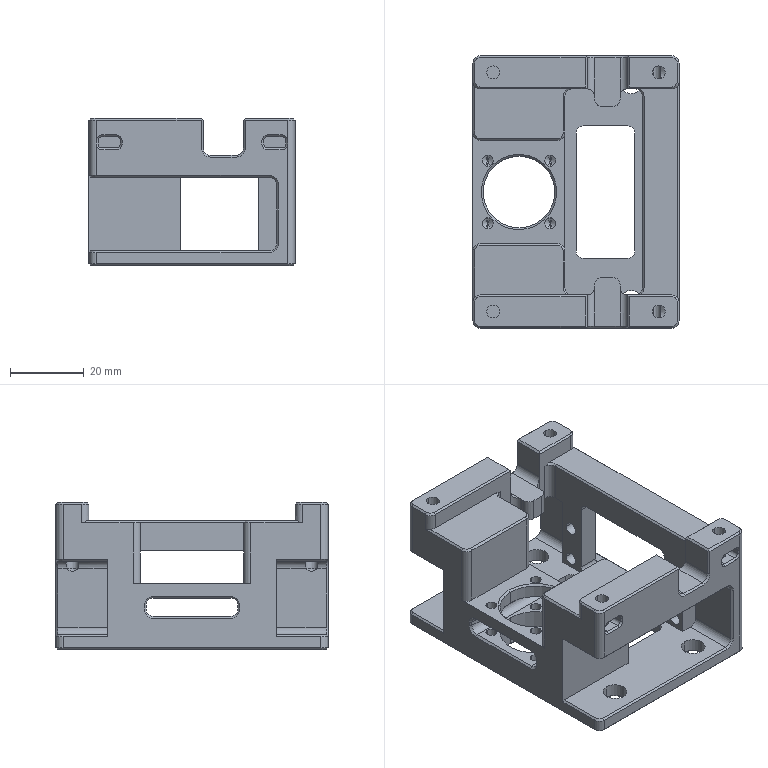NC program | Mastercam | posted with a generic post | part box 56 x 74 x 40 mm
Lines 1 to 1578 of 45205, first 1423 of 1578 lines:
%
:0001()
(MATERIAL - ALUMINUM MM - 2024)
(T24|100 FEM |H24)
(T11|12 FEM |H11|XY STOCK TO LEAVE - .15|Z STOCK TO LEAVE - 0.)
(T12|12 FEM |H12)
(T8|8 FEM |H8|XY STOCK TO LEAVE - .07|Z STOCK TO LEAVE - 0.)
(T4|4 FEM |H4|XY STOCK TO LEAVE - .1|Z STOCK TO LEAVE - 0.)
(T5|4 CHM |H5)
(T3|3 FEM |H3)
(T2|2 FEM |H2|XY STOCK TO LEAVE - 0.|Z STOCK TO LEAVE - .05)
(T18|4 BM/BNOS |H18)
(T6|6 FEM |H6|XY STOCK TO LEAVE - -.03|Z STOCK TO LEAVE - 0.)
N100 G21
N102 G0 G17 G40 G80 G90 G94 G98
N104 G0 G28 G91 Z0.
N106 G0 G28 X0. Y0.
(100 FEM |TOOL - 24|DIA. OFF. - 24|LEN. - 24|TOOL DIA. - 100.)
N108 T24 M6
N110 G0 G54 G90 X-121. Y0. C0. B0. S4000 M3
N112 G43 H24 Z50.
N114 Z2.
N116 G1 Z0. F600.
N118 X121. F1000.
N120 G0 Z50.
N122 M5
N124 G0 G28 G91 Z0.
N126 G28
N128 M01
N130 G0 G17 G40 G80 G90 G94 G98
N132 G0 G28 G91 Z0.
(12 FEM |TOOL - 11|DIA. OFF. - 11|LEN. - 11|TOOL DIA. - 12.)
N134 T11 M6
N136 G0 G54 G90 X36.2 Y-41.35 C0. B0. S10000 M3
N138 G43 H11 Z50.
N140 Z1.
N142 G1 Z0. F600.
N144 Y-35.35 F5000.
N146 G3 X35. Y-34.15 I-1.2
N148 G1 X-35. Z-.237
N150 G2 X-43.15 Y-26. Z-.28 J8.15
N152 G1 Y26. Z-.457
N154 G2 X-35. Y34.15 Z-.5 I8.15
N156 G1 X35. Z-.737
N158 G2 X43.15 Y26. Z-.78 J-8.15
N160 G1 Y-26. Z-.957
N162 G2 X35. Y-34.15 Z-1. I-8.15
N164 G1 X-35. Z-1.237
N166 G2 X-43.15 Y-26. Z-1.28 J8.15
N168 G1 Y26. Z-1.457
N170 G2 X-35. Y34.15 Z-1.5 I8.15
N172 G1 X35. Z-1.737
N174 G2 X43.15 Y26. Z-1.78 J-8.15
N176 G1 Y-26. Z-1.957
N178 G2 X35. Y-34.15 Z-2. I-8.15
N180 G1 X-35. Z-2.237
N182 G2 X-43.15 Y-26. Z-2.28 J8.15
N184 G1 Y26. Z-2.457
N186 G2 X-35. Y34.15 Z-2.5 I8.15
N188 G1 X35. Z-2.737
N190 G2 X43.15 Y26. Z-2.78 J-8.15
N192 G1 Y-26. Z-2.957
N194 G2 X35. Y-34.15 Z-3. I-8.15
N196 G1 X-35. Z-3.237
N198 G2 X-43.15 Y-26. Z-3.28 J8.15
N200 G1 Y26. Z-3.457
N202 G2 X-35. Y34.15 Z-3.5 I8.15
N204 G1 X35. Z-3.737
N206 G2 X43.15 Y26. Z-3.78 J-8.15
N208 G1 Y-26. Z-3.957
N210 G2 X35. Y-34.15 Z-4. I-8.15
N212 G1 X-35. Z-4.237
N214 G2 X-43.15 Y-26. Z-4.28 J8.15
N216 G1 Y26. Z-4.457
N218 G2 X-35. Y34.15 Z-4.5 I8.15
N220 G1 X35. Z-4.737
N222 G2 X43.15 Y26. Z-4.78 J-8.15
N224 G1 Y-26. Z-4.957
N226 G2 X35. Y-34.15 Z-5. I-8.15
N228 G1 X-35. Z-5.237
N230 G2 X-43.15 Y-26. Z-5.28 J8.15
N232 G1 Y26. Z-5.457
N234 G2 X-35. Y34.15 Z-5.5 I8.15
N236 G1 X35. Z-5.737
N238 G2 X43.15 Y26. Z-5.78 J-8.15
N240 G1 Y-26. Z-5.957
N242 G2 X35. Y-34.15 Z-6. I-8.15
N244 G1 X-35. Z-6.237
N246 G2 X-43.15 Y-26. Z-6.28 J8.15
N248 G1 Y26. Z-6.457
N250 G2 X-35. Y34.15 Z-6.5 I8.15
N252 G1 X35. Z-6.737
N254 G2 X43.15 Y26. Z-6.78 J-8.15
N256 G1 Y-26. Z-6.957
N258 G2 X35. Y-34.15 Z-7. I-8.15
N260 G1 X-35. Z-7.237
N262 G2 X-43.15 Y-26. Z-7.28 J8.15
N264 G1 Y26. Z-7.457
N266 G2 X-35. Y34.15 Z-7.5 I8.15
N268 G1 X35. Z-7.737
N270 G2 X43.15 Y26. Z-7.78 J-8.15
N272 G1 Y-26. Z-7.957
N274 G2 X35. Y-34.15 Z-8. I-8.15
N276 G1 X-35. Z-8.237
N278 G2 X-43.15 Y-26. Z-8.28 J8.15
N280 G1 Y26. Z-8.457
N282 G2 X-35. Y34.15 Z-8.5 I8.15
N284 G1 X35. Z-8.737
N286 G2 X43.15 Y26. Z-8.78 J-8.15
N288 G1 Y-26. Z-8.957
N290 G2 X35. Y-34.15 Z-9. I-8.15
N292 G1 X-35. Z-9.237
N294 G2 X-43.15 Y-26. Z-9.28 J8.15
N296 G1 Y26. Z-9.457
N298 G2 X-35. Y34.15 Z-9.5 I8.15
N300 G1 X35. Z-9.737
N302 G2 X43.15 Y26. Z-9.78 J-8.15
N304 G1 Y-26. Z-9.957
N306 G2 X35. Y-34.15 Z-10. I-8.15
N308 G1 X-35. Z-10.237
N310 G2 X-43.15 Y-26. Z-10.28 J8.15
N312 G1 Y26. Z-10.457
N314 G2 X-35. Y34.15 Z-10.5 I8.15
N316 G1 X35. Z-10.737
N318 G2 X43.15 Y26. Z-10.78 J-8.15
N320 G1 Y-26. Z-10.957
N322 G2 X35. Y-34.15 Z-11. I-8.15
N324 G1 X-35. Z-11.237
N326 G2 X-43.15 Y-26. Z-11.28 J8.15
N328 G1 Y26. Z-11.457
N330 G2 X-35. Y34.15 Z-11.5 I8.15
N332 G1 X35. Z-11.737
N334 G2 X43.15 Y26. Z-11.78 J-8.15
N336 G1 Y-26. Z-11.957
N338 G2 X35. Y-34.15 Z-12. I-8.15
N340 G1 X-35. Z-12.237
N342 G2 X-43.15 Y-26. Z-12.28 J8.15
N344 G1 Y26. Z-12.457
N346 G2 X-35. Y34.15 Z-12.5 I8.15
N348 G1 X35. Z-12.737
N350 G2 X43.15 Y26. Z-12.78 J-8.15
N352 G1 Y-26. Z-12.957
N354 G2 X35. Y-34.15 Z-13. I-8.15
N356 G1 X-35. Z-13.237
N358 G2 X-43.15 Y-26. Z-13.28 J8.15
N360 G1 Y26. Z-13.457
N362 G2 X-35. Y34.15 Z-13.5 I8.15
N364 G1 X35. Z-13.737
N366 G2 X43.15 Y26. Z-13.78 J-8.15
N368 G1 Y-26. Z-13.957
N370 G2 X35. Y-34.15 Z-14. I-8.15
N372 G1 X-35. Z-14.237
N374 G2 X-43.15 Y-26. Z-14.28 J8.15
N376 G1 Y26. Z-14.457
N378 G2 X-35. Y34.15 Z-14.5 I8.15
N380 G1 X35. Z-14.737
N382 G2 X43.15 Y26. Z-14.78 J-8.15
N384 G1 Y-26. Z-14.957
N386 G2 X35. Y-34.15 Z-15. I-8.15
N388 G1 X-35. Z-15.237
N390 G2 X-43.15 Y-26. Z-15.28 J8.15
N392 G1 Y26. Z-15.457
N394 G2 X-35. Y34.15 Z-15.5 I8.15
N396 G1 X35. Z-15.737
N398 G2 X43.15 Y26. Z-15.78 J-8.15
N400 G1 Y-26. Z-15.957
N402 G2 X35. Y-34.15 Z-16. I-8.15
N404 G1 X-35. Z-16.237
N406 G2 X-43.15 Y-26. Z-16.28 J8.15
N408 G1 Y26. Z-16.457
N410 G2 X-35. Y34.15 Z-16.5 I8.15
N412 G1 X35. Z-16.737
N414 G2 X43.15 Y26. Z-16.78 J-8.15
N416 G1 Y-26. Z-16.957
N418 G2 X35. Y-34.15 Z-17. I-8.15
N420 G1 X-35. Z-17.237
N422 G2 X-43.15 Y-26. Z-17.28 J8.15
N424 G1 Y26. Z-17.457
N426 G2 X-35. Y34.15 Z-17.5 I8.15
N428 G1 X35. Z-17.737
N430 G2 X43.15 Y26. Z-17.78 J-8.15
N432 G1 Y-26. Z-17.957
N434 G2 X35. Y-34.15 Z-18. I-8.15
N436 G1 X-35. Z-18.237
N438 G2 X-43.15 Y-26. Z-18.28 J8.15
N440 G1 Y26. Z-18.457
N442 G2 X-35. Y34.15 Z-18.5 I8.15
N444 G1 X35. Z-18.737
N446 G2 X43.15 Y26. Z-18.78 J-8.15
N448 G1 Y-26. Z-18.957
N450 G2 X35. Y-34.15 Z-19. I-8.15
N452 G1 X-35. Z-19.237
N454 G2 X-43.15 Y-26. Z-19.28 J8.15
N456 G1 Y26. Z-19.457
N458 G2 X-35. Y34.15 Z-19.5 I8.15
N460 G1 X35. Z-19.737
N462 G2 X43.15 Y26. Z-19.78 J-8.15
N464 G1 Y-26. Z-19.957
N466 G2 X35. Y-34.15 Z-20. I-8.15
N468 G1 X-35. Z-20.237
N470 G2 X-43.15 Y-26. Z-20.28 J8.15
N472 G1 Y26. Z-20.457
N474 G2 X-35. Y34.15 Z-20.5 I8.15
N476 G1 X35. Z-20.737
N478 G2 X43.15 Y26. Z-20.78 J-8.15
N480 G1 Y-26. Z-20.957
N482 G2 X35. Y-34.15 Z-21. I-8.15
N484 G1 X-35. Z-21.237
N486 G2 X-43.15 Y-26. Z-21.28 J8.15
N488 G1 Y26. Z-21.457
N490 G2 X-35. Y34.15 Z-21.5 I8.15
N492 G1 X35. Z-21.737
N494 G2 X43.15 Y26. Z-21.78 J-8.15
N496 G1 Y-26. Z-21.957
N498 G2 X35. Y-34.15 Z-22. I-8.15
N500 G1 X-35. Z-22.237
N502 G2 X-43.15 Y-26. Z-22.28 J8.15
N504 G1 Y26. Z-22.457
N506 G2 X-35. Y34.15 Z-22.5 I8.15
N508 G1 X35. Z-22.737
N510 G2 X43.15 Y26. Z-22.78 J-8.15
N512 G1 Y-26. Z-22.957
N514 G2 X35. Y-34.15 Z-23. I-8.15
N516 G1 X-35. Z-23.237
N518 G2 X-43.15 Y-26. Z-23.28 J8.15
N520 G1 Y26. Z-23.457
N522 G2 X-35. Y34.15 Z-23.5 I8.15
N524 G1 X35. Z-23.737
N526 G2 X43.15 Y26. Z-23.78 J-8.15
N528 G1 Y-26. Z-23.957
N530 G2 X35. Y-34.15 Z-24. I-8.15
N532 G1 X-35. Z-24.237
N534 G2 X-43.15 Y-26. Z-24.28 J8.15
N536 G1 Y26. Z-24.457
N538 G2 X-35. Y34.15 Z-24.5 I8.15
N540 G1 X35. Z-24.737
N542 G2 X43.15 Y26. Z-24.78 J-8.15
N544 G1 Y-26. Z-24.957
N546 G2 X35. Y-34.15 Z-25. I-8.15
N548 G1 X-35. Z-25.237
N550 G2 X-43.15 Y-26. Z-25.28 J8.15
N552 G1 Y26. Z-25.457
N554 G2 X-35. Y34.15 Z-25.5 I8.15
N556 G1 X35. Z-25.737
N558 G2 X43.15 Y26. Z-25.78 J-8.15
N560 G1 Y-26. Z-25.957
N562 G2 X35. Y-34.15 Z-26. I-8.15
N564 G1 X-35. Z-26.237
N566 G2 X-43.15 Y-26. Z-26.28 J8.15
N568 G1 Y26. Z-26.457
N570 G2 X-35. Y34.15 Z-26.5 I8.15
N572 G1 X35. Z-26.737
N574 G2 X43.15 Y26. Z-26.78 J-8.15
N576 G1 Y-26. Z-26.957
N578 G2 X35. Y-34.15 Z-27. I-8.15
N580 G1 X-35. Z-27.237
N582 G2 X-43.15 Y-26. Z-27.28 J8.15
N584 G1 Y26. Z-27.457
N586 G2 X-35. Y34.15 Z-27.5 I8.15
N588 G1 X35. Z-27.737
N590 G2 X43.15 Y26. Z-27.78 J-8.15
N592 G1 Y-26. Z-27.957
N594 G2 X35. Y-34.15 Z-28. I-8.15
N596 G1 X-35. Z-28.237
N598 G2 X-43.15 Y-26. Z-28.28 J8.15
N600 G1 Y26. Z-28.457
N602 G2 X-35. Y34.15 Z-28.5 I8.15
N604 G1 X35. Z-28.737
N606 G2 X43.15 Y26. Z-28.78 J-8.15
N608 G1 Y-26. Z-28.957
N610 G2 X35. Y-34.15 Z-29. I-8.15
N612 G1 X-35. Z-29.237
N614 G2 X-43.15 Y-26. Z-29.28 J8.15
N616 G1 Y26. Z-29.457
N618 G2 X-35. Y34.15 Z-29.5 I8.15
N620 G1 X35. Z-29.737
N622 G2 X43.15 Y26. Z-29.78 J-8.15
N624 G1 Y-26. Z-29.957
N626 G2 X35. Y-34.15 Z-30. I-8.15
N628 G1 X-35. Z-30.237
N630 G2 X-43.15 Y-26. Z-30.28 J8.15
N632 G1 Y26. Z-30.457
N634 G2 X-35. Y34.15 Z-30.5 I8.15
N636 G1 X35. Z-30.737
N638 G2 X43.15 Y26. Z-30.78 J-8.15
N640 G1 Y-26. Z-30.957
N642 G2 X35. Y-34.15 Z-31. I-8.15
N644 G1 X-35. Z-31.237
N646 G2 X-43.15 Y-26. Z-31.28 J8.15
N648 G1 Y26. Z-31.457
N650 G2 X-35. Y34.15 Z-31.5 I8.15
N652 G1 X35. Z-31.737
N654 G2 X43.15 Y26. Z-31.78 J-8.15
N656 G1 Y-26. Z-31.957
N658 G2 X35. Y-34.15 Z-32. I-8.15
N660 G1 X-35. Z-32.237
N662 G2 X-43.15 Y-26. Z-32.28 J8.15
N664 G1 Y26. Z-32.457
N666 G2 X-35. Y34.15 Z-32.5 I8.15
N668 G1 X35. Z-32.737
N670 G2 X43.15 Y26. Z-32.78 J-8.15
N672 G1 Y-26. Z-32.957
N674 G2 X35. Y-34.15 Z-33. I-8.15
N676 G1 X-35. Z-33.237
N678 G2 X-43.15 Y-26. Z-33.28 J8.15
N680 G1 Y26. Z-33.457
N682 G2 X-35. Y34.15 Z-33.5 I8.15
N684 G1 X35. Z-33.737
N686 G2 X43.15 Y26. Z-33.78 J-8.15
N688 G1 Y-26. Z-33.957
N690 G2 X35. Y-34.15 Z-34. I-8.15
N692 G1 X-35. Z-34.237
N694 G2 X-43.15 Y-26. Z-34.28 J8.15
N696 G1 Y26. Z-34.457
N698 G2 X-35. Y34.15 Z-34.5 I8.15
N700 G1 X35. Z-34.737
N702 G2 X43.15 Y26. Z-34.78 J-8.15
N704 G1 Y-26. Z-34.957
N706 G2 X35. Y-34.15 Z-35. I-8.15
N708 G1 X-35. Z-35.237
N710 G2 X-43.15 Y-26. Z-35.28 J8.15
N712 G1 Y26. Z-35.457
N714 G2 X-35. Y34.15 Z-35.5 I8.15
N716 G1 X35. Z-35.737
N718 G2 X43.15 Y26. Z-35.78 J-8.15
N720 G1 Y-26. Z-35.957
N722 G2 X35. Y-34.15 Z-36. I-8.15
N724 G1 X-35. Z-36.237
N726 G2 X-43.15 Y-26. Z-36.28 J8.15
N728 G1 Y26. Z-36.457
N730 G2 X-35. Y34.15 Z-36.5 I8.15
N732 G1 X35. Z-36.737
N734 G2 X43.15 Y26. Z-36.78 J-8.15
N736 G1 Y-26. Z-36.957
N738 G2 X35. Y-34.15 Z-37. I-8.15
N740 G1 X-35. Z-37.237
N742 G2 X-43.15 Y-26. Z-37.28 J8.15
N744 G1 Y26. Z-37.457
N746 G2 X-35. Y34.15 Z-37.5 I8.15
N748 G1 X35. Z-37.737
N750 G2 X43.15 Y26. Z-37.78 J-8.15
N752 G1 Y-26. Z-37.957
N754 G2 X35. Y-34.15 Z-38. I-8.15
N756 G1 X-35. Z-38.237
N758 G2 X-43.15 Y-26. Z-38.28 J8.15
N760 G1 Y26. Z-38.457
N762 G2 X-35. Y34.15 Z-38.5 I8.15
N764 G1 X35. Z-38.737
N766 G2 X43.15 Y26. Z-38.78 J-8.15
N768 G1 Y-26. Z-38.957
N770 G2 X35. Y-34.15 Z-39. I-8.15
N772 G1 X-35. Z-39.237
N774 G2 X-43.15 Y-26. Z-39.28 J8.15
N776 G1 Y26. Z-39.457
N778 G2 X-35. Y34.15 Z-39.5 I8.15
N780 G1 X35. Z-39.737
N782 G2 X43.15 Y26. Z-39.78 J-8.15
N784 G1 Y-26. Z-39.957
N786 G2 X35. Y-34.15 Z-40. I-8.15
N788 G1 X-35. Z-40.237
N790 G2 X-43.15 Y-26. Z-40.28 J8.15
N792 G1 Y26. Z-40.457
N794 G2 X-35. Y34.15 Z-40.5 I8.15
N796 G1 X35.
N798 G2 X43.15 Y26. J-8.15
N800 G1 Y-26.
N802 G2 X35. Y-34.15 I-8.15
N804 G1 X-35.
N806 G2 X-43.15 Y-26. J8.15
N808 G1 Y26.
N810 G2 X-35. Y34.15 I8.15
N812 G1 X-34.499
N814 G3 X-33.299 Y35.35 J1.2
N816 G1 Y41.35
N818 G0 Z50.
N820 M5
N822 G0 G28 G91 Z0.
N824 G28
N826 M01
N828 G0 G17 G40 G80 G90 G94 G98
N830 G0 G28 G91 Z0.
(12 FEM |TOOL - 12|DIA. OFF. - 12|LEN. - 12|TOOL DIA. - 12.)
N832 T12 M6
N834 G0 G54 G90 X40.525 Y-36.27 C0. B0. S7000 M3
N836 G43 H12 Z50.
N838 Z1.
N840 G1 Z-20.25 F600.
N842 X39.612 Y-34.051 F1000.
N844 G3 X38.502 Y-33.307 I-1.11 J-.456
N846 X38.045 Y-33.398 J-1.2
N848 G2 X35. Y-34. I-3.045 J7.398
N850 G1 X-35.
N852 G2 X-43. Y-26. J8.
N854 G1 Y26.
N856 G2 X-35. Y34. I8.
N858 G1 X35.
N860 G2 X43. Y26. J-8.
N862 G1 Y-26.
N864 G2 X38.045 Y-33.398 I-8.
N866 X37.577 Y-33.574 I-3.045 J7.398
N868 G3 X36.764 Y-34.71 I.387 J-1.136
N870 X36.828 Y-35.096 I1.2
N872 G1 X37.601 Y-37.368
N874 X40.525 Y-36.27
N876 Z-40.5 F600.
N878 X39.612 Y-34.051 F1000.
N880 G3 X38.502 Y-33.307 I-1.11 J-.456
N882 X38.045 Y-33.398 J-1.2
N884 G2 X35. Y-34. I-3.045 J7.398
N886 G1 X-35.
N888 G2 X-43. Y-26. J8.
N890 G1 Y26.
N892 G2 X-35. Y34. I8.
N894 G1 X35.
N896 G2 X43. Y26. J-8.
N898 G1 Y-26.
N900 G2 X38.045 Y-33.398 I-8.
N902 X37.577 Y-33.574 I-3.045 J7.398
N904 G3 X36.764 Y-34.71 I.387 J-1.136
N906 X36.828 Y-35.096 I1.2
N908 G1 X37.601 Y-37.368
N910 G0 Z50.
N912 M5
N914 G0 G28 G91 Z0.
N916 G28
N918 M01
N920 G0 G17 G40 G80 G90 G94 G98
N922 G0 G28 G91 Z0.
(12 FEM |TOOL - 11|DIA. OFF. - 11|LEN. - 11|TOOL DIA. - 12.)
N924 T11 M6
N926 G0 G54 G90 X3.65 Y15.5 C0. B0. S7000 M3
N928 G43 H11 Z50.
N930 Z1.
N932 G1 Z0. F600.
N934 G3 X0. Y19.15 Z-.125 I-3.65 F2000.
N936 X-3.65 Y15.5 Z-.25 J-3.65
N938 X0. Y11.85 Z-.375 I3.65
N940 X3.65 Y15.5 Z-.5 J3.65
N942 X0. Y19.15 Z-.625 I-3.65
N944 X-3.65 Y15.5 Z-.75 J-3.65
N946 X0. Y11.85 Z-.875 I3.65
N948 X3.65 Y15.5 Z-1. J3.65
N950 X0. Y19.15 Z-1.125 I-3.65
N952 X-3.65 Y15.5 Z-1.25 J-3.65
N954 X0. Y11.85 Z-1.375 I3.65
N956 X3.65 Y15.5 Z-1.5 J3.65
N958 X0. Y19.15 Z-1.625 I-3.65
N960 X-3.65 Y15.5 Z-1.75 J-3.65
N962 X0. Y11.85 Z-1.875 I3.65
N964 X3.65 Y15.5 Z-2. J3.65
N966 X0. Y19.15 Z-2.125 I-3.65
N968 X-3.65 Y15.5 Z-2.25 J-3.65
N970 X0. Y11.85 Z-2.375 I3.65
N972 X3.65 Y15.5 Z-2.5 J3.65
N974 X0. Y19.15 Z-2.625 I-3.65
N976 X-3.65 Y15.5 Z-2.75 J-3.65
N978 X0. Y11.85 Z-2.875 I3.65
N980 X3.65 Y15.5 Z-3. J3.65
N982 X0. Y19.15 Z-3.125 I-3.65
N984 X-3.65 Y15.5 Z-3.25 J-3.65
N986 X0. Y11.85 Z-3.375 I3.65
N988 X3.65 Y15.5 Z-3.5 J3.65
N990 X0. Y19.15 Z-3.625 I-3.65
N992 X-3.65 Y15.5 Z-3.75 J-3.65
N994 X0. Y11.85 Z-3.875 I3.65
N996 X3.65 Y15.5 Z-4. J3.65
N998 X0. Y19.15 Z-4.125 I-3.65
N1000 X-3.65 Y15.5 Z-4.25 J-3.65
N1002 X0. Y11.85 Z-4.375 I3.65
N1004 X3.65 Y15.5 Z-4.5 J3.65
N1006 X0. Y19.15 Z-4.625 I-3.65
N1008 X-3.65 Y15.5 Z-4.75 J-3.65
N1010 X0. Y11.85 Z-4.875 I3.65
N1012 X3.65 Y15.5 Z-5. J3.65
N1014 X0. Y19.15 Z-5.125 I-3.65
N1016 X-3.65 Y15.5 Z-5.25 J-3.65
N1018 X0. Y11.85 Z-5.375 I3.65
N1020 X3.65 Y15.5 Z-5.5 J3.65
N1022 X0. Y19.15 Z-5.625 I-3.65
N1024 X-3.65 Y15.5 Z-5.75 J-3.65
N1026 X0. Y11.85 Z-5.875 I3.65
N1028 X3.65 Y15.5 Z-6. J3.65
N1030 X0. Y19.15 Z-6.125 I-3.65
N1032 X-3.65 Y15.5 Z-6.25 J-3.65
N1034 X0. Y11.85 Z-6.375 I3.65
N1036 X3.65 Y15.5 Z-6.5 J3.65
N1038 X0. Y19.15 Z-6.625 I-3.65
N1040 X-3.65 Y15.5 Z-6.75 J-3.65
N1042 X0. Y11.85 Z-6.875 I3.65
N1044 X3.65 Y15.5 Z-7. J3.65
N1046 X0. Y19.15 Z-7.125 I-3.65
N1048 X-3.65 Y15.5 Z-7.25 J-3.65
N1050 X0. Y11.85 Z-7.375 I3.65
N1052 X3.65 Y15.5 Z-7.5 J3.65
N1054 X0. Y19.15 Z-7.625 I-3.65
N1056 X-3.65 Y15.5 Z-7.75 J-3.65
N1058 X0. Y11.85 Z-7.875 I3.65
N1060 X3.65 Y15.5 Z-8. J3.65
N1062 X0. Y19.15 Z-8.125 I-3.65
N1064 X-3.65 Y15.5 Z-8.25 J-3.65
N1066 X0. Y11.85 Z-8.375 I3.65
N1068 X3.65 Y15.5 Z-8.5 J3.65
N1070 X0. Y19.15 Z-8.625 I-3.65
N1072 X-3.65 Y15.5 Z-8.75 J-3.65
N1074 X0. Y11.85 Z-8.875 I3.65
N1076 X3.65 Y15.5 Z-9. J3.65
N1078 X0. Y19.15 Z-9.125 I-3.65
N1080 X-3.65 Y15.5 Z-9.25 J-3.65
N1082 X0. Y11.85 Z-9.375 I3.65
N1084 X3.65 Y15.5 Z-9.5 J3.65
N1086 X0. Y19.15 Z-9.625 I-3.65
N1088 X-3.65 Y15.5 Z-9.75 J-3.65
N1090 X0. Y11.85 Z-9.875 I3.65
N1092 X3.65 Y15.5 Z-10. J3.65
N1094 X0. Y19.15 Z-10.125 I-3.65
N1096 X-3.65 Y15.5 Z-10.25 J-3.65
N1098 X0. Y11.85 Z-10.375 I3.65
N1100 X3.65 Y15.5 Z-10.5 J3.65
N1102 X0. Y19.15 Z-10.625 I-3.65
N1104 X-3.65 Y15.5 Z-10.75 J-3.65
N1106 X0. Y11.85 Z-10.875 I3.65
N1108 X3.65 Y15.5 Z-11. J3.65
N1110 X0. Y19.15 Z-11.125 I-3.65
N1112 X-3.65 Y15.5 Z-11.25 J-3.65
N1114 X0. Y11.85 Z-11.375 I3.65
N1116 X3.65 Y15.5 Z-11.5 J3.65
N1118 X0. Y19.15 Z-11.625 I-3.65
N1120 X-3.65 Y15.5 Z-11.75 J-3.65
N1122 X0. Y11.85 Z-11.875 I3.65
N1124 X3.65 Y15.5 Z-12. J3.65
N1126 X0. Y19.15 Z-12.125 I-3.65
N1128 X-3.65 Y15.5 Z-12.25 J-3.65
N1130 X0. Y11.85 Z-12.375 I3.65
N1132 X3.65 Y15.5 Z-12.5 J3.65
N1134 X0. Y19.15 Z-12.625 I-3.65
N1136 X-3.65 Y15.5 Z-12.75 J-3.65
N1138 X0. Y11.85 Z-12.875 I3.65
N1140 X3.65 Y15.5 Z-13. J3.65
N1142 X0. Y19.15 Z-13.125 I-3.65
N1144 X-3.65 Y15.5 Z-13.25 J-3.65
N1146 X0. Y11.85 Z-13.375 I3.65
N1148 X3.65 Y15.5 Z-13.5 J3.65
N1150 X0. Y19.15 Z-13.625 I-3.65
N1152 X-3.65 Y15.5 Z-13.75 J-3.65
N1154 X0. Y11.85 Z-13.875 I3.65
N1156 X3.65 Y15.5 Z-14. J3.65
N1158 X0. Y19.15 Z-14.125 I-3.65
N1160 X-3.65 Y15.5 Z-14.25 J-3.65
N1162 X0. Y11.85 Z-14.375 I3.65
N1164 X3.65 Y15.5 Z-14.5 J3.65
N1166 X0. Y19.15 Z-14.625 I-3.65
N1168 X-3.65 Y15.5 Z-14.75 J-3.65
N1170 X0. Y11.85 Z-14.875 I3.65
N1172 X3.65 Y15.5 Z-15. J3.65
N1174 X0. Y19.15 Z-15.125 I-3.65
N1176 X-3.65 Y15.5 Z-15.25 J-3.65
N1178 X0. Y11.85 Z-15.375 I3.65
N1180 X3.65 Y15.5 Z-15.5 J3.65
N1182 X0. Y19.15 Z-15.625 I-3.65
N1184 X-3.65 Y15.5 Z-15.75 J-3.65
N1186 X0. Y11.85 Z-15.875 I3.65
N1188 X3.65 Y15.5 Z-16. J3.65
N1190 X0. Y19.15 Z-16.125 I-3.65
N1192 X-3.65 Y15.5 Z-16.25 J-3.65
N1194 X0. Y11.85 Z-16.375 I3.65
N1196 X3.65 Y15.5 Z-16.5 J3.65
N1198 X0. Y19.15 Z-16.625 I-3.65
N1200 X-3.65 Y15.5 Z-16.75 J-3.65
N1202 X0. Y11.85 Z-16.875 I3.65
N1204 X3.65 Y15.5 Z-17. J3.65
N1206 X0. Y19.15 Z-17.125 I-3.65
N1208 X-3.65 Y15.5 Z-17.25 J-3.65
N1210 X0. Y11.85 Z-17.375 I3.65
N1212 X3.65 Y15.5 Z-17.5 J3.65
N1214 X0. Y19.15 Z-17.625 I-3.65
N1216 X-3.65 Y15.5 Z-17.75 J-3.65
N1218 X0. Y11.85 Z-17.875 I3.65
N1220 X3.65 Y15.5 Z-18. J3.65
N1222 X0. Y19.15 Z-18.125 I-3.65
N1224 X-3.65 Y15.5 Z-18.25 J-3.65
N1226 X0. Y11.85 Z-18.375 I3.65
N1228 X3.65 Y15.5 Z-18.5 J3.65
N1230 X0. Y19.15 Z-18.625 I-3.65
N1232 X-3.65 Y15.5 Z-18.75 J-3.65
N1234 X0. Y11.85 Z-18.875 I3.65
N1236 X3.65 Y15.5 Z-19. J3.65
N1238 X0. Y19.15 Z-19.125 I-3.65
N1240 X-3.65 Y15.5 Z-19.25 J-3.65
N1242 X0. Y11.85 Z-19.375 I3.65
N1244 X3.65 Y15.5 Z-19.5 J3.65
N1246 X0. Y19.15 Z-19.625 I-3.65
N1248 X-3.65 Y15.5 Z-19.75 J-3.65
N1250 X0. Y11.85 Z-19.875 I3.65
N1252 X3.65 Y15.5 Z-20. J3.65
N1254 X0. Y19.15 I-3.65
N1256 X-3.65 Y15.5 J-3.65
N1258 X0. Y11.85 I3.65
N1260 X3.65 Y15.5 J3.65
N1262 X3.616 Y15.999 I-3.65
N1264 G0 Z50.
N1266 M5
N1268 G0 G28 G91 Z0.
N1270 G28
N1272 M01
N1274 G0 G17 G40 G80 G90 G94 G98
N1276 G0 G28 G91 Z0.
(12 FEM |TOOL - 12|DIA. OFF. - 12|LEN. - 12|TOOL DIA. - 12.)
N1278 T12 M6
N1280 G0 G54 G90 X1.315 Y14.3 C0. B0. S7000 M3
N1282 G43 H12 Z50.
N1284 Z1.
N1286 G1 Z-20. F600.
N1288 X2.515 F1000.
N1290 G3 X3.715 Y15.5 J1.2
N1292 X0. Y19.215 I-3.715
N1294 X-3.715 Y15.5 J-3.715
N1296 X0. Y11.785 I3.715
N1298 X3.715 Y15.5 J3.715
N1300 X3.681 Y15.998 I-3.715
N1302 X2.492 Y17.037 I-1.189 J-.161
N1304 X2.331 Y17.027 J-1.2
N1306 G1 X1.142 Y16.866
N1308 X1.365 Y14.3
N1310 X2.565
N1312 G3 X3.765 Y15.5 J1.2
N1314 X0. Y19.265 I-3.765
N1316 X-3.765 Y15.5 J-3.765
N1318 X0. Y11.735 I3.765
N1320 X3.765 Y15.5 J3.765
N1322 X3.732 Y15.999 I-3.765
N1324 X2.542 Y17.041 I-1.19 J-.159
N1326 G1 X2.463 Y17.038
N1328 X2.384 Y17.03
N1330 X1.194 Y16.87
N1332 G0 Z50.
N1334 M5
N1336 G0 G28 G91 Z0.
N1338 G28
N1340 M01
N1342 G0 G17 G40 G80 G90 G94 G98
N1344 G0 G28 G91 Z0.
(8 FEM |TOOL - 8|DIA. OFF. - 8|LEN. - 8|TOOL DIA. - 8.)
N1346 T8 M6
N1348 G0 G54 G90 X13.93 Y-4.07 C0. B0. S7000 M3
N1350 G43 H8 Z50.
N1352 Z1.
N1354 G1 Z0. F600.
N1356 X-13.93 Z-.156 F2000.
N1358 Y-11.93 Z-.2
N1360 X13.93 Z-.356
N1362 Y-4.07 Z-.4
N1364 X-13.93 Z-.556
N1366 Y-11.93 Z-.6
N1368 X13.93 Z-.756
N1370 Y-4.07 Z-.8
N1372 X-13.93 Z-.956
N1374 Y-11.93 Z-1.
N1376 X13.93 Z-1.156
N1378 Y-4.07 Z-1.2
N1380 X-13.93 Z-1.356
N1382 Y-11.93 Z-1.4
N1384 X13.93 Z-1.556
N1386 Y-4.07 Z-1.6
N1388 X-13.93 Z-1.756
N1390 Y-11.93 Z-1.8
N1392 X13.93 Z-1.956
N1394 Y-4.07 Z-2.
N1396 X-13.93 Z-2.156
N1398 Y-11.93 Z-2.2
N1400 X13.93 Z-2.356
N1402 Y-4.07 Z-2.4
N1404 X-13.93 Z-2.556
N1406 Y-11.93 Z-2.6
N1408 X13.93 Z-2.756
N1410 Y-4.07 Z-2.8
N1412 X-13.93 Z-2.956
N1414 Y-11.93 Z-3.
N1416 X13.93 Z-3.156
N1418 Y-4.07 Z-3.2
N1420 X-13.93 Z-3.356
N1422 Y-11.93 Z-3.4
N1424 X13.93 Z-3.556
N1426 Y-4.07 Z-3.6
N1428 X-13.93 Z-3.756
N1430 Y-11.93 Z-3.8
N1432 X13.93 Z-3.956
N1434 Y-4.07 Z-4.
N1436 X-13.93 Z-4.156
N1438 Y-11.93 Z-4.2
N1440 X13.93 Z-4.356
N1442 Y-4.07 Z-4.4
N1444 X-13.93 Z-4.556
N1446 Y-11.93 Z-4.6
N1448 X13.93 Z-4.756
N1450 Y-4.07 Z-4.8
N1452 X-13.93 Z-4.956
N1454 Y-11.93 Z-5.
N1456 X13.93
N1458 Y-4.07
N1460 X-13.93
N1462 Y-11.93
N1464 X-13.429
N1466 G0 Z50.
N1468 M5
N1470 G0 G28 G91 Z0.
N1472 G28
N1474 M01
N1476 G0 G17 G40 G80 G90 G94 G98
N1478 G0 G28 G91 Z0.
(4 FEM |TOOL - 4|DIA. OFF. - 4|LEN. - 4|TOOL DIA. - 4.)
N1480 T4 M6
N1482 G0 G54 G90 X-10.532 Y-2.9 C0. B0. S7000 M3
N1484 G43 H4 Z50.
N1486 Z1.
N1488 G1 Z-.5 F600.
N1490 Y-2.5 F3000.
N1492 G3 X-10.932 Y-2.1 I-.4
N1494 G1 X-15.9
N1496 Y-6.988
N1498 G3 X-15.5 Y-7.388 I.4
N1500 G1 X-15.1
N1502 X-10.532 Y-2.9
N1504 Z-1. F600.
N1506 Y-2.5 F3000.
N1508 G3 X-10.932 Y-2.1 I-.4
N1510 G1 X-15.9
N1512 Y-6.988
N1514 G3 X-15.5 Y-7.388 I.4
N1516 G1 X-15.1
N1518 X-10.532 Y-2.9
N1520 Z-1.5 F600.
N1522 Y-2.5 F3000.
N1524 G3 X-10.932 Y-2.1 I-.4
N1526 G1 X-15.9
N1528 Y-6.988
N1530 G3 X-15.5 Y-7.388 I.4
N1532 G1 X-15.1
N1534 X-10.532 Y-2.9
N1536 Z-2. F600.
N1538 Y-2.5 F3000.
N1540 G3 X-10.932 Y-2.1 I-.4
N1542 G1 X-15.9
N1544 Y-6.988
N1546 G3 X-15.5 Y-7.388 I.4
N1548 G1 X-15.1
N1550 X-10.532 Y-2.9
N1552 Z-2.5 F600.
N1554 Y-2.5 F3000.
N1556 G3 X-10.932 Y-2.1 I-.4
N1558 G1 X-15.9
N1560 Y-6.988
N1562 G3 X-15.5 Y-7.388 I.4
N1564 G1 X-15.1
N1566 X-10.532 Y-2.9
N1568 Z-3. F600.
N1570 Y-2.5 F3000.
N1572 G3 X-10.932 Y-2.1 I-.4
N1574 G1 X-15.9
N1576 Y-6.988
N1578 G3 X-15.5 Y-7.388 I.4
N1580 G1 X-15.1
N1582 X-10.532 Y-2.9
N1584 Z-3.5 F600.
N1586 Y-2.5 F3000.
N1588 G3 X-10.932 Y-2.1 I-.4
N1590 G1 X-15.9
N1592 Y-6.988
N1594 G3 X-15.5 Y-7.388 I.4
N1596 G1 X-15.1
N1598 X-10.532 Y-2.9
N1600 Z-4. F600.
N1602 Y-2.5 F3000.
N1604 G3 X-10.932 Y-2.1 I-.4
N1606 G1 X-15.9
N1608 Y-6.988
N1610 G3 X-15.5 Y-7.388 I.4
N1612 G1 X-15.1
N1614 X-10.532 Y-2.9
N1616 Z-4.5 F600.
N1618 Y-2.5 F3000.
N1620 G3 X-10.932 Y-2.1 I-.4
N1622 G1 X-15.9
N1624 Y-6.988
N1626 G3 X-15.5 Y-7.388 I.4
N1628 G1 X-15.1
N1630 X-10.532 Y-2.9
N1632 Z-5. F600.
N1634 Y-2.5 F3000.
N1636 G3 X-10.932 Y-2.1 I-.4
N1638 G1 X-15.9
N1640 Y-6.988
N1642 G3 X-15.5 Y-7.388 I.4
N1644 G1 X-15.1
N1646 G0 Z50.
N1648 Y-8.598
N1650 Z1.
N1652 G1 Z-.5 F600.
N1654 X-15.5 F3000.
N1656 G3 X-15.9 Y-8.998 J-.4
N1658 G1 Y-13.9
N1660 X-10.666
N1662 G3 X-10.266 Y-13.5 J.4
N1664 G1 Y-13.1
N1666 X-15.1 Y-8.598
N1668 Z-1. F600.
N1670 X-15.5 F3000.
N1672 G3 X-15.9 Y-8.998 J-.4
N1674 G1 Y-13.9
N1676 X-10.666
N1678 G3 X-10.266 Y-13.5 J.4
N1680 G1 Y-13.1
N1682 X-15.1 Y-8.598
N1684 Z-1.5 F600.
N1686 X-15.5 F3000.
N1688 G3 X-15.9 Y-8.998 J-.4
N1690 G1 Y-13.9
N1692 X-10.666
N1694 G3 X-10.266 Y-13.5 J.4
N1696 G1 Y-13.1
N1698 X-15.1 Y-8.598
N1700 Z-2. F600.
N1702 X-15.5 F3000.
N1704 G3 X-15.9 Y-8.998 J-.4
N1706 G1 Y-13.9
N1708 X-10.666
N1710 G3 X-10.266 Y-13.5 J.4
N1712 G1 Y-13.1
N1714 X-15.1 Y-8.598
N1716 Z-2.5 F600.
N1718 X-15.5 F3000.
N1720 G3 X-15.9 Y-8.998 J-.4
N1722 G1 Y-13.9
N1724 X-10.666
N1726 G3 X-10.266 Y-13.5 J.4
N1728 G1 Y-13.1
N1730 X-15.1 Y-8.598
N1732 Z-3. F600.
N1734 X-15.5 F3000.
N1736 G3 X-15.9 Y-8.998 J-.4
N1738 G1 Y-13.9
N1740 X-10.666
N1742 G3 X-10.266 Y-13.5 J.4
N1744 G1 Y-13.1
N1746 X-15.1 Y-8.598
N1748 Z-3.5 F600.
N1750 X-15.5 F3000.
N1752 G3 X-15.9 Y-8.998 J-.4
N1754 G1 Y-13.9
N1756 X-10.666
N1758 G3 X-10.266 Y-13.5 J.4
N1760 G1 Y-13.1
N1762 X-15.1 Y-8.598
N1764 Z-4. F600.
N1766 X-15.5 F3000.
N1768 G3 X-15.9 Y-8.998 J-.4
N1770 G1 Y-13.9
N1772 X-10.666
N1774 G3 X-10.266 Y-13.5 J.4
N1776 G1 Y-13.1
N1778 X-15.1 Y-8.598
N1780 Z-4.5 F600.
N1782 X-15.5 F3000.
N1784 G3 X-15.9 Y-8.998 J-.4
N1786 G1 Y-13.9
N1788 X-10.666
N1790 G3 X-10.266 Y-13.5 J.4
N1792 G1 Y-13.1
N1794 X-15.1 Y-8.598
N1796 Z-5. F600.
N1798 X-15.5 F3000.
N1800 G3 X-15.9 Y-8.998 J-.4
N1802 G1 Y-13.9
N1804 X-10.666
N1806 G3 X-10.266 Y-13.5 J.4
N1808 G1 Y-13.1
N1810 G0 Z50.
N1812 X10.266
N1814 Z1.
N1816 G1 Z-.5 F600.
N1818 Y-13.5 F3000.
N1820 G3 X10.666 Y-13.9 I.4
N1822 G1 X15.9
N1824 Y-8.997
N1826 G3 X15.5 Y-8.597 I-.4
N1828 G1 X15.1
N1830 X10.266 Y-13.1
N1832 Z-1. F600.
N1834 Y-13.5 F3000.
N1836 G3 X10.666 Y-13.9 I.4
N1838 G1 X15.9
N1840 Y-8.997
N1842 G3 X15.5 Y-8.597 I-.4
N1844 G1 X15.1
N1846 X10.266 Y-13.1
N1848 Z-1.5 F600.
N1850 Y-13.5 F3000.
N1852 G3 X10.666 Y-13.9 I.4
N1854 G1 X15.9
N1856 Y-8.997
N1858 G3 X15.5 Y-8.597 I-.4
N1860 G1 X15.1
N1862 X10.266 Y-13.1
N1864 Z-2. F600.
N1866 Y-13.5 F3000.
N1868 G3 X10.666 Y-13.9 I.4
N1870 G1 X15.9
N1872 Y-8.997
N1874 G3 X15.5 Y-8.597 I-.4
N1876 G1 X15.1
N1878 X10.266 Y-13.1
N1880 Z-2.5 F600.
N1882 Y-13.5 F3000.
N1884 G3 X10.666 Y-13.9 I.4
N1886 G1 X15.9
N1888 Y-8.997
N1890 G3 X15.5 Y-8.597 I-.4
N1892 G1 X15.1
N1894 X10.266 Y-13.1
N1896 Z-3. F600.
N1898 Y-13.5 F3000.
N1900 G3 X10.666 Y-13.9 I.4
N1902 G1 X15.9
N1904 Y-8.997
N1906 G3 X15.5 Y-8.597 I-.4
N1908 G1 X15.1
N1910 X10.266 Y-13.1
N1912 Z-3.5 F600.
N1914 Y-13.5 F3000.
N1916 G3 X10.666 Y-13.9 I.4
N1918 G1 X15.9
N1920 Y-8.997
N1922 G3 X15.5 Y-8.597 I-.4
N1924 G1 X15.1
N1926 X10.266 Y-13.1
N1928 Z-4. F600.
N1930 Y-13.5 F3000.
N1932 G3 X10.666 Y-13.9 I.4
N1934 G1 X15.9
N1936 Y-8.997
N1938 G3 X15.5 Y-8.597 I-.4
N1940 G1 X15.1
N1942 X10.266 Y-13.1
N1944 Z-4.5 F600.
N1946 Y-13.5 F3000.
N1948 G3 X10.666 Y-13.9 I.4
N1950 G1 X15.9
N1952 Y-8.997
N1954 G3 X15.5 Y-8.597 I-.4
N1956 G1 X15.1
N1958 X10.266 Y-13.1
N1960 Z-5. F600.
N1962 Y-13.5 F3000.
N1964 G3 X10.666 Y-13.9 I.4
N1966 G1 X15.9
N1968 Y-8.997
N1970 G3 X15.5 Y-8.597 I-.4
N1972 G1 X15.1
N1974 G0 Z50.
N1976 Y-7.388
N1978 Z1.
N1980 G1 Z-.5 F600.
N1982 X15.5 F3000.
N1984 G3 X15.9 Y-6.988 J.4
N1986 G1 Y-2.1
N1988 X10.922
N1990 G3 X10.522 Y-2.5 J-.4
N1992 G1 Y-2.9
N1994 X15.1 Y-7.388
N1996 Z-1. F600.
N1998 X15.5 F3000.
N2000 G3 X15.9 Y-6.988 J.4
N2002 G1 Y-2.1
N2004 X10.922
N2006 G3 X10.522 Y-2.5 J-.4
N2008 G1 Y-2.9
N2010 X15.1 Y-7.388
N2012 Z-1.5 F600.
N2014 X15.5 F3000.
N2016 G3 X15.9 Y-6.988 J.4
N2018 G1 Y-2.1
N2020 X10.922
N2022 G3 X10.522 Y-2.5 J-.4
N2024 G1 Y-2.9
N2026 X15.1 Y-7.388
N2028 Z-2. F600.
N2030 X15.5 F3000.
N2032 G3 X15.9 Y-6.988 J.4
N2034 G1 Y-2.1
N2036 X10.922
N2038 G3 X10.522 Y-2.5 J-.4
N2040 G1 Y-2.9
N2042 X15.1 Y-7.388
N2044 Z-2.5 F600.
N2046 X15.5 F3000.
N2048 G3 X15.9 Y-6.988 J.4
N2050 G1 Y-2.1
N2052 X10.922
N2054 G3 X10.522 Y-2.5 J-.4
N2056 G1 Y-2.9
N2058 X15.1 Y-7.388
N2060 Z-3. F600.
N2062 X15.5 F3000.
N2064 G3 X15.9 Y-6.988 J.4
N2066 G1 Y-2.1
N2068 X10.922
N2070 G3 X10.522 Y-2.5 J-.4
N2072 G1 Y-2.9
N2074 X15.1 Y-7.388
N2076 Z-3.5 F600.
N2078 X15.5 F3000.
N2080 G3 X15.9 Y-6.988 J.4
N2082 G1 Y-2.1
N2084 X10.922
N2086 G3 X10.522 Y-2.5 J-.4
N2088 G1 Y-2.9
N2090 X15.1 Y-7.388
N2092 Z-4. F600.
N2094 X15.5 F3000.
N2096 G3 X15.9 Y-6.988 J.4
N2098 G1 Y-2.1
N2100 X10.922
N2102 G3 X10.522 Y-2.5 J-.4
N2104 G1 Y-2.9
N2106 X15.1 Y-7.388
N2108 Z-4.5 F600.
N2110 X15.5 F3000.
N2112 G3 X15.9 Y-6.988 J.4
N2114 G1 Y-2.1
N2116 X10.922
N2118 G3 X10.522 Y-2.5 J-.4
N2120 G1 Y-2.9
N2122 X15.1 Y-7.388
N2124 Z-5. F600.
N2126 X15.5 F3000.
N2128 G3 X15.9 Y-6.988 J.4
N2130 G1 Y-2.1
N2132 X10.922
N2134 G3 X10.522 Y-2.5 J-.4
N2136 G1 Y-2.9
N2138 G0 Z50.
N2140 X16. Y-1.99
N2142 Z1.
N2144 G1 Z-5. F600.
N2146 X-16. F1000.
N2148 G3 X-16.01 Y-2. J-.01
N2150 G1 Y-14.
N2152 G3 X-16. Y-14.01 I.01
N2154 G1 X16.
N2156 G3 X16.01 Y-14. J.01
N2158 G1 Y-2.
N2160 G3 X16. Y-1.99 I-.01
N2162 G1 X15.5
N2164 G3 X15.1 Y-2.39 J-.4
N2166 G1 Y-2.79
N2168 G0 Z50.
N2170 X-28.82 Y15.
N2172 Z1.
N2174 G1 Z0. F600.
N2176 G3 X-30. Y16.18 Z-.075 I-1.18 F2000.
N2178 X-31.18 Y15. Z-.15 J-1.18
N2180 X-30. Y13.82 Z-.225 I1.18
N2182 X-28.82 Y15. Z-.3 J1.18
N2184 X-30. Y16.18 Z-.375 I-1.18
N2186 X-31.18 Y15. Z-.45 J-1.18
N2188 X-30. Y13.82 Z-.525 I1.18
N2190 X-28.82 Y15. Z-.6 J1.18
N2192 X-30. Y16.18 Z-.675 I-1.18
N2194 X-31.18 Y15. Z-.75 J-1.18
N2196 X-30. Y13.82 Z-.825 I1.18
N2198 X-28.82 Y15. Z-.9 J1.18
N2200 X-30. Y16.18 Z-.975 I-1.18
N2202 X-31.18 Y15. Z-1.05 J-1.18
N2204 X-30. Y13.82 Z-1.125 I1.18
N2206 X-28.82 Y15. Z-1.2 J1.18
N2208 X-30. Y16.18 Z-1.275 I-1.18
N2210 X-31.18 Y15. Z-1.35 J-1.18
N2212 X-30. Y13.82 Z-1.425 I1.18
N2214 X-28.82 Y15. Z-1.5 J1.18
N2216 X-30. Y16.18 Z-1.575 I-1.18
N2218 X-31.18 Y15. Z-1.65 J-1.18
N2220 X-30. Y13.82 Z-1.725 I1.18
N2222 X-28.82 Y15. Z-1.8 J1.18
N2224 X-30. Y16.18 Z-1.875 I-1.18
N2226 X-31.18 Y15. Z-1.95 J-1.18
N2228 X-30. Y13.82 Z-2.025 I1.18
N2230 X-28.82 Y15. Z-2.1 J1.18
N2232 X-30. Y16.18 Z-2.175 I-1.18
N2234 X-31.18 Y15. Z-2.25 J-1.18
N2236 X-30. Y13.82 Z-2.325 I1.18
N2238 X-28.82 Y15. Z-2.4 J1.18
N2240 X-30. Y16.18 Z-2.475 I-1.18
N2242 X-31.18 Y15. Z-2.55 J-1.18
N2244 X-30. Y13.82 Z-2.625 I1.18
N2246 X-28.82 Y15. Z-2.7 J1.18
N2248 X-30. Y16.18 Z-2.775 I-1.18
N2250 X-31.18 Y15. Z-2.85 J-1.18
N2252 X-30. Y13.82 Z-2.925 I1.18
N2254 X-28.82 Y15. Z-3. J1.18
N2256 X-30. Y16.18 Z-3.075 I-1.18
N2258 X-31.18 Y15. Z-3.15 J-1.18
N2260 X-30. Y13.82 Z-3.225 I1.18
N2262 X-28.82 Y15. Z-3.3 J1.18
N2264 X-30. Y16.18 Z-3.375 I-1.18
N2266 X-31.18 Y15. Z-3.45 J-1.18
N2268 X-30. Y13.82 Z-3.525 I1.18
N2270 X-28.82 Y15. Z-3.6 J1.18
N2272 X-30. Y16.18 Z-3.675 I-1.18
N2274 X-31.18 Y15. Z-3.75 J-1.18
N2276 X-30. Y13.82 Z-3.825 I1.18
N2278 X-28.82 Y15. Z-3.9 J1.18
N2280 X-30. Y16.18 Z-3.975 I-1.18
N2282 X-31.18 Y15. Z-4.05 J-1.18
N2284 X-30. Y13.82 Z-4.125 I1.18
N2286 X-28.82 Y15. Z-4.2 J1.18
N2288 X-30. Y16.18 Z-4.275 I-1.18
N2290 X-31.18 Y15. Z-4.35 J-1.18
N2292 X-30. Y13.82 Z-4.425 I1.18
N2294 X-28.82 Y15. Z-4.5 J1.18
N2296 X-30. Y16.18 Z-4.575 I-1.18
N2298 X-31.18 Y15. Z-4.65 J-1.18
N2300 X-30. Y13.82 Z-4.725 I1.18
N2302 X-28.82 Y15. Z-4.8 J1.18
N2304 X-30. Y16.18 Z-4.875 I-1.18
N2306 X-31.18 Y15. Z-4.95 J-1.18
N2308 X-30.59 Y13.978 Z-5. I1.18
N2310 X-30. Y13.82 I.59 J1.022
N2312 X-28.82 Y15. J1.18
N2314 X-30. Y16.18 I-1.18
N2316 X-31.18 Y15. J-1.18
N2318 X-30.118 Y13.826 I1.18
N2320 G0 Z50.
N2322 X-28.82 Y-15.
N2324 Z1.
N2326 G1 Z0. F600.
N2328 G3 X-30. Y-13.82 Z-.075 I-1.18 F2000.
N2330 X-31.18 Y-15. Z-.15 J-1.18
N2332 X-30. Y-16.18 Z-.225 I1.18
N2334 X-28.82 Y-15. Z-.3 J1.18
N2336 X-30. Y-13.82 Z-.375 I-1.18
N2338 X-31.18 Y-15. Z-.45 J-1.18
N2340 X-30. Y-16.18 Z-.525 I1.18
N2342 X-28.82 Y-15. Z-.6 J1.18
N2344 X-30. Y-13.82 Z-.675 I-1.18
N2346 X-31.18 Y-15. Z-.75 J-1.18
N2348 X-30. Y-16.18 Z-.825 I1.18
N2350 X-28.82 Y-15. Z-.9 J1.18
N2352 X-30. Y-13.82 Z-.975 I-1.18
N2354 X-31.18 Y-15. Z-1.05 J-1.18
N2356 X-30. Y-16.18 Z-1.125 I1.18
N2358 X-28.82 Y-15. Z-1.2 J1.18
N2360 X-30. Y-13.82 Z-1.275 I-1.18
N2362 X-31.18 Y-15. Z-1.35 J-1.18
N2364 X-30. Y-16.18 Z-1.425 I1.18
N2366 X-28.82 Y-15. Z-1.5 J1.18
N2368 X-30. Y-13.82 Z-1.575 I-1.18
N2370 X-31.18 Y-15. Z-1.65 J-1.18
N2372 X-30. Y-16.18 Z-1.725 I1.18
N2374 X-28.82 Y-15. Z-1.8 J1.18
N2376 X-30. Y-13.82 Z-1.875 I-1.18
N2378 X-31.18 Y-15. Z-1.95 J-1.18
N2380 X-30. Y-16.18 Z-2.025 I1.18
N2382 X-28.82 Y-15. Z-2.1 J1.18
N2384 X-30. Y-13.82 Z-2.175 I-1.18
N2386 X-31.18 Y-15. Z-2.25 J-1.18
N2388 X-30. Y-16.18 Z-2.325 I1.18
N2390 X-28.82 Y-15. Z-2.4 J1.18
N2392 X-30. Y-13.82 Z-2.475 I-1.18
N2394 X-31.18 Y-15. Z-2.55 J-1.18
N2396 X-30. Y-16.18 Z-2.625 I1.18
N2398 X-28.82 Y-15. Z-2.7 J1.18
N2400 X-30. Y-13.82 Z-2.775 I-1.18
N2402 X-31.18 Y-15. Z-2.85 J-1.18
N2404 X-30. Y-16.18 Z-2.925 I1.18
N2406 X-28.82 Y-15. Z-3. J1.18
N2408 X-30. Y-13.82 Z-3.075 I-1.18
N2410 X-31.18 Y-15. Z-3.15 J-1.18
N2412 X-30. Y-16.18 Z-3.225 I1.18
N2414 X-28.82 Y-15. Z-3.3 J1.18
N2416 X-30. Y-13.82 Z-3.375 I-1.18
N2418 X-31.18 Y-15. Z-3.45 J-1.18
N2420 X-30. Y-16.18 Z-3.525 I1.18
N2422 X-28.82 Y-15. Z-3.6 J1.18
N2424 X-30. Y-13.82 Z-3.675 I-1.18
N2426 X-31.18 Y-15. Z-3.75 J-1.18
N2428 X-30. Y-16.18 Z-3.825 I1.18
N2430 X-28.82 Y-15. Z-3.9 J1.18
N2432 X-30. Y-13.82 Z-3.975 I-1.18
N2434 X-31.18 Y-15. Z-4.05 J-1.18
N2436 X-30. Y-16.18 Z-4.125 I1.18
N2438 X-28.82 Y-15. Z-4.2 J1.18
N2440 X-30. Y-13.82 Z-4.275 I-1.18
N2442 X-31.18 Y-15. Z-4.35 J-1.18
N2444 X-30. Y-16.18 Z-4.425 I1.18
N2446 X-28.82 Y-15. Z-4.5 J1.18
N2448 X-30. Y-13.82 Z-4.575 I-1.18
N2450 X-31.18 Y-15. Z-4.65 J-1.18
N2452 X-30. Y-16.18 Z-4.725 I1.18
N2454 X-28.82 Y-15. Z-4.8 J1.18
N2456 X-30. Y-13.82 Z-4.875 I-1.18
N2458 X-31.18 Y-15. Z-4.95 J-1.18
N2460 X-30.59 Y-16.022 Z-5. I1.18
N2462 X-30. Y-16.18 I.59 J1.022
N2464 X-28.82 Y-15. J1.18
N2466 X-30. Y-13.82 I-1.18
N2468 X-31.18 Y-15. J-1.18
N2470 X-30.118 Y-16.174 I1.18
N2472 G0 Z50.
N2474 X31.18 Y-15.
N2476 Z1.
N2478 G1 Z0. F600.
N2480 G3 X30. Y-13.82 Z-.075 I-1.18 F2000.
N2482 X28.82 Y-15. Z-.15 J-1.18
N2484 X30. Y-16.18 Z-.225 I1.18
N2486 X31.18 Y-15. Z-.3 J1.18
N2488 X30. Y-13.82 Z-.375 I-1.18
N2490 X28.82 Y-15. Z-.45 J-1.18
N2492 X30. Y-16.18 Z-.525 I1.18
N2494 X31.18 Y-15. Z-.6 J1.18
N2496 X30. Y-13.82 Z-.675 I-1.18
N2498 X28.82 Y-15. Z-.75 J-1.18
N2500 X30. Y-16.18 Z-.825 I1.18
N2502 X31.18 Y-15. Z-.9 J1.18
N2504 X30. Y-13.82 Z-.975 I-1.18
N2506 X28.82 Y-15. Z-1.05 J-1.18
N2508 X30. Y-16.18 Z-1.125 I1.18
N2510 X31.18 Y-15. Z-1.2 J1.18
N2512 X30. Y-13.82 Z-1.275 I-1.18
N2514 X28.82 Y-15. Z-1.35 J-1.18
N2516 X30. Y-16.18 Z-1.425 I1.18
N2518 X31.18 Y-15. Z-1.5 J1.18
N2520 X30. Y-13.82 Z-1.575 I-1.18
N2522 X28.82 Y-15. Z-1.65 J-1.18
N2524 X30. Y-16.18 Z-1.725 I1.18
N2526 X31.18 Y-15. Z-1.8 J1.18
N2528 X30. Y-13.82 Z-1.875 I-1.18
N2530 X28.82 Y-15. Z-1.95 J-1.18
N2532 X30. Y-16.18 Z-2.025 I1.18
N2534 X31.18 Y-15. Z-2.1 J1.18
N2536 X30. Y-13.82 Z-2.175 I-1.18
N2538 X28.82 Y-15. Z-2.25 J-1.18
N2540 X30. Y-16.18 Z-2.325 I1.18
N2542 X31.18 Y-15. Z-2.4 J1.18
N2544 X30. Y-13.82 Z-2.475 I-1.18
N2546 X28.82 Y-15. Z-2.55 J-1.18
N2548 X30. Y-16.18 Z-2.625 I1.18
N2550 X31.18 Y-15. Z-2.7 J1.18
N2552 X30. Y-13.82 Z-2.775 I-1.18
N2554 X28.82 Y-15. Z-2.85 J-1.18
N2556 X30. Y-16.18 Z-2.925 I1.18
N2558 X31.18 Y-15. Z-3. J1.18
N2560 X30. Y-13.82 Z-3.075 I-1.18
N2562 X28.82 Y-15. Z-3.15 J-1.18
N2564 X30. Y-16.18 Z-3.225 I1.18
N2566 X31.18 Y-15. Z-3.3 J1.18
N2568 X30. Y-13.82 Z-3.375 I-1.18
N2570 X28.82 Y-15. Z-3.45 J-1.18
N2572 X30. Y-16.18 Z-3.525 I1.18
N2574 X31.18 Y-15. Z-3.6 J1.18
N2576 X30. Y-13.82 Z-3.675 I-1.18
N2578 X28.82 Y-15. Z-3.75 J-1.18
N2580 X30. Y-16.18 Z-3.825 I1.18
N2582 X31.18 Y-15. Z-3.9 J1.18
N2584 X30. Y-13.82 Z-3.975 I-1.18
N2586 X28.82 Y-15. Z-4.05 J-1.18
N2588 X30. Y-16.18 Z-4.125 I1.18
N2590 X31.18 Y-15. Z-4.2 J1.18
N2592 X30. Y-13.82 Z-4.275 I-1.18
N2594 X28.82 Y-15. Z-4.35 J-1.18
N2596 X30. Y-16.18 Z-4.425 I1.18
N2598 X31.18 Y-15. Z-4.5 J1.18
N2600 X30. Y-13.82 Z-4.575 I-1.18
N2602 X28.82 Y-15. Z-4.65 J-1.18
N2604 X30. Y-16.18 Z-4.725 I1.18
N2606 X31.18 Y-15. Z-4.8 J1.18
N2608 X30. Y-13.82 Z-4.875 I-1.18
N2610 X28.82 Y-15. Z-4.95 J-1.18
N2612 X29.41 Y-16.022 Z-5. I1.18
N2614 X30. Y-16.18 I.59 J1.022
N2616 X31.18 Y-15. J1.18
N2618 X30. Y-13.82 I-1.18
N2620 X28.82 Y-15. J-1.18
N2622 X29.882 Y-16.174 I1.18
N2624 G0 Z50.
N2626 X31.18 Y15.
N2628 Z1.
N2630 G1 Z0. F600.
N2632 G3 X30. Y16.18 Z-.075 I-1.18 F2000.
N2634 X28.82 Y15. Z-.15 J-1.18
N2636 X30. Y13.82 Z-.225 I1.18
N2638 X31.18 Y15. Z-.3 J1.18
N2640 X30. Y16.18 Z-.375 I-1.18
N2642 X28.82 Y15. Z-.45 J-1.18
N2644 X30. Y13.82 Z-.525 I1.18
N2646 X31.18 Y15. Z-.6 J1.18
N2648 X30. Y16.18 Z-.675 I-1.18
N2650 X28.82 Y15. Z-.75 J-1.18
N2652 X30. Y13.82 Z-.825 I1.18
N2654 X31.18 Y15. Z-.9 J1.18
N2656 X30. Y16.18 Z-.975 I-1.18
N2658 X28.82 Y15. Z-1.05 J-1.18
N2660 X30. Y13.82 Z-1.125 I1.18
N2662 X31.18 Y15. Z-1.2 J1.18
N2664 X30. Y16.18 Z-1.275 I-1.18
N2666 X28.82 Y15. Z-1.35 J-1.18
N2668 X30. Y13.82 Z-1.425 I1.18
N2670 X31.18 Y15. Z-1.5 J1.18
N2672 X30. Y16.18 Z-1.575 I-1.18
N2674 X28.82 Y15. Z-1.65 J-1.18
N2676 X30. Y13.82 Z-1.725 I1.18
N2678 X31.18 Y15. Z-1.8 J1.18
N2680 X30. Y16.18 Z-1.875 I-1.18
N2682 X28.82 Y15. Z-1.95 J-1.18
N2684 X30. Y13.82 Z-2.025 I1.18
N2686 X31.18 Y15. Z-2.1 J1.18
N2688 X30. Y16.18 Z-2.175 I-1.18
N2690 X28.82 Y15. Z-2.25 J-1.18
N2692 X30. Y13.82 Z-2.325 I1.18
N2694 X31.18 Y15. Z-2.4 J1.18
N2696 X30. Y16.18 Z-2.475 I-1.18
N2698 X28.82 Y15. Z-2.55 J-1.18
N2700 X30. Y13.82 Z-2.625 I1.18
N2702 X31.18 Y15. Z-2.7 J1.18
N2704 X30. Y16.18 Z-2.775 I-1.18
N2706 X28.82 Y15. Z-2.85 J-1.18
N2708 X30. Y13.82 Z-2.925 I1.18
N2710 X31.18 Y15. Z-3. J1.18
N2712 X30. Y16.18 Z-3.075 I-1.18
N2714 X28.82 Y15. Z-3.15 J-1.18
N2716 X30. Y13.82 Z-3.225 I1.18
N2718 X31.18 Y15. Z-3.3 J1.18
N2720 X30. Y16.18 Z-3.375 I-1.18
N2722 X28.82 Y15. Z-3.45 J-1.18
N2724 X30. Y13.82 Z-3.525 I1.18
N2726 X31.18 Y15. Z-3.6 J1.18
N2728 X30. Y16.18 Z-3.675 I-1.18
N2730 X28.82 Y15. Z-3.75 J-1.18
N2732 X30. Y13.82 Z-3.825 I1.18
N2734 X31.18 Y15. Z-3.9 J1.18
N2736 X30. Y16.18 Z-3.975 I-1.18
N2738 X28.82 Y15. Z-4.05 J-1.18
N2740 X30. Y13.82 Z-4.125 I1.18
N2742 X31.18 Y15. Z-4.2 J1.18
N2744 X30. Y16.18 Z-4.275 I-1.18
N2746 X28.82 Y15. Z-4.35 J-1.18
N2748 X30. Y13.82 Z-4.425 I1.18
N2750 X31.18 Y15. Z-4.5 J1.18
N2752 X30. Y16.18 Z-4.575 I-1.18
N2754 X28.82 Y15. Z-4.65 J-1.18
N2756 X30. Y13.82 Z-4.725 I1.18
N2758 X31.18 Y15. Z-4.8 J1.18
N2760 X30. Y16.18 Z-4.875 I-1.18
N2762 X28.82 Y15. Z-4.95 J-1.18
N2764 X29.41 Y13.978 Z-5. I1.18
N2766 X30. Y13.82 I.59 J1.022
N2768 X31.18 Y15. J1.18
N2770 X30. Y16.18 I-1.18
N2772 X28.82 Y15. J-1.18
N2774 X29.882 Y13.826 I1.18
N2776 G0 Z50.
N2778 X-29.56 Y14.6
N2780 Z1.
N2782 G1 Z-5. F600.
N2784 X-29.16 F1000.
N2786 G3 X-28.76 Y15. J.4
N2788 X-30. Y16.24 I-1.24
N2790 X-31.24 Y15. J-1.24
N2792 X-30. Y13.76 I1.24
N2794 X-28.76 Y15. J1.24
N2796 X-28.859 Y15.487 I-1.24
N2798 X-29.227 Y15.73 I-.368 J-.157
N2800 X-29.384 Y15.698 J-.4
N2802 G1 X-29.752 Y15.541
N2804 X-29.51 Y14.6
N2806 X-29.11
N2808 G3 X-28.71 Y15. J.4
N2810 X-30. Y16.29 I-1.29
N2812 X-31.29 Y15. J-1.29
N2814 X-30. Y13.71 I1.29
N2816 X-28.71 Y15. J1.29
N2818 X-28.806 Y15.488 I-1.29
N2820 X-29.176 Y15.736 I-.37 J-.152
N2822 X-29.327 Y15.707 J-.4
N2824 G1 X-29.698 Y15.556
N2826 G0 Z50.
N2828 X-29.56 Y-15.4
N2830 Z1.
N2832 G1 Z-5. F600.
N2834 X-29.16 F1000.
N2836 G3 X-28.76 Y-15. J.4
N2838 X-30. Y-13.76 I-1.24
N2840 X-31.24 Y-15. J-1.24
N2842 X-30. Y-16.24 I1.24
N2844 X-28.76 Y-15. J1.24
N2846 X-28.859 Y-14.513 I-1.24
N2848 X-29.227 Y-14.27 I-.368 J-.157
N2850 X-29.384 Y-14.302 J-.4
N2852 G1 X-29.752 Y-14.459
N2854 X-29.51 Y-15.4
N2856 X-29.11
N2858 G3 X-28.71 Y-15. J.4
N2860 X-30. Y-13.71 I-1.29
N2862 X-31.29 Y-15. J-1.29
N2864 X-30. Y-16.29 I1.29
N2866 X-28.71 Y-15. J1.29
N2868 X-28.806 Y-14.512 I-1.29
N2870 X-29.176 Y-14.264 I-.37 J-.152
N2872 X-29.327 Y-14.293 J-.4
N2874 G1 X-29.698 Y-14.444
N2876 G0 Z50.
N2878 X30.44 Y-15.4
N2880 Z1.
N2882 G1 Z-5. F600.
N2884 X30.84 F1000.
N2886 G3 X31.24 Y-15. J.4
N2888 X30. Y-13.76 I-1.24
N2890 X28.76 Y-15. J-1.24
N2892 X30. Y-16.24 I1.24
N2894 X31.24 Y-15. J1.24
N2896 X31.141 Y-14.513 I-1.24
N2898 X30.773 Y-14.27 I-.368 J-.157
N2900 X30.616 Y-14.302 J-.4
N2902 G1 X30.248 Y-14.459
N2904 X30.49 Y-15.4